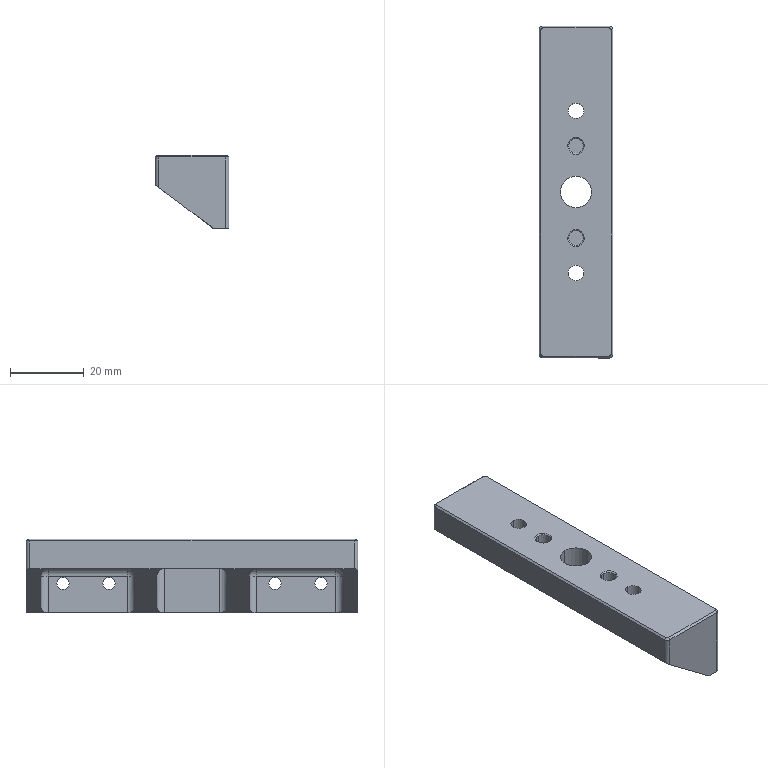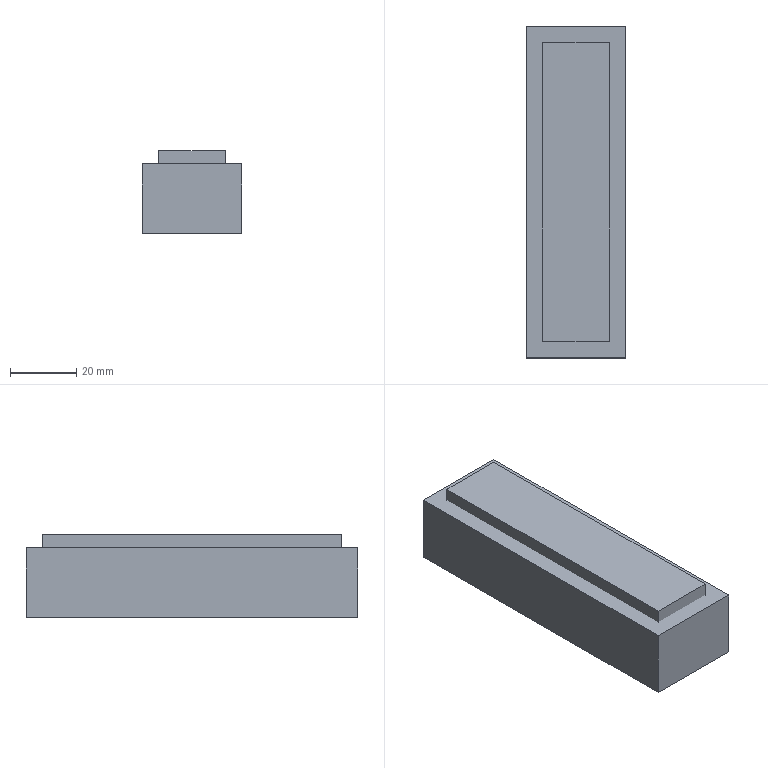CAM job | NX | 3+2 milling, drilling | part box 20 x 90 x 20 mm | stock box 30 x 100 x 25 mm
Tools:
number,name,description,diameter,corner_radius,flute_length,length,flutes
19,D80,Milling Tool-5 Parameters,80.0,0.0,50.0,75.0,2
1,D6A45,Milling Tool-5 Parameters,6.0,0.0,50.0,75.0,2
4,4.2ZT,Drilling Tool,4.2,0.0,35.0,50.0,2
15,D10,Milling Tool-5 Parameters,10.0,0.0,50.0,75.0,2
14,D10JING,Milling Tool-5 Parameters,10.0,0.0,50.0,75.0,2
12,D6,Milling Tool-5 Parameters,6.0,0.0,50.0,75.0,2
17,D3,Milling Tool-5 Parameters,3.0,0.0,50.0,75.0,2
18,D4R0.5,Milling Tool-5 Parameters,4.0,0.5,50.0,75.0,2
3,3.3ZT,Drilling Tool,3.3,0.0,35.0,50.0,2
Operations:
program,operation,operation_type,tool,method,geometry_group,spindle_rpm,surface_speed,feed_per_tooth,feed_cut,feed_plunge,cut_length_mm,path_length_mm,cut_time_min,machine_time_min
1,FLOOR_WALL,VolumeBased25DMillingOperation,D80,METHOD,A,6500.0,1633.0,0.1154,1500.0,100.0,192.0,246.0,0.128,0.1334
1,DRILLING_COPY_1,Operation,D6A45,METHOD,A,5000.0,94.0,0.035,350.0,0.0,26.5,170.635,0.0757,0.0901
1,DRILLING_COPY_COPY,Operation,4.2ZT,METHOD,A,2000.0,20.0,0.045,180.0,0.0,30.524,168.149,0.1696,0.1833
1,ADAPTIVE_MILLING,CavityMilling,D10,METHOD,A,9500.0,298.0,0.1579,3000.0,1000.0,1321.539,1415.539,0.4425,0.4519
1,ZLEVEL_PROFILE_COPY_1_COPY_COPY_1,ZLevelMilling,D10JING,METHOD,A,9500.0,298.0,0.0632,1200.0,1000.0,257.063,355.063,0.2148,0.2246
1,HOLE_MILLING,CylinderMilling,D6,METHOD,A,9500.0,179.0,0.0789,1500.0,100.0,145.569,213.069,0.097,0.1038
1,HOLE_MILLING_COPY,CylinderMilling,D3,METHOD,A,9500.0,89.0,0.0632,1200.0,100.0,138.875,294.875,0.1157,0.1313
1,PLANAR_MILL_COPY_COPY_COPY_COPY_COPY_COPY_1,PlanarMilling,D6A45,METHOD,A,9500.0,179.0,0.0658,1250.0,100.0,225.891,284.891,0.1807,0.1866
1,HOLE_MILLING_COPY_COPY,CylinderMilling,D3,METHOD,A,9500.0,89.0,0.0632,1200.0,100.0,26.316,182.316,0.0219,0.0375
2,FLOOR_WALL_COPY,VolumeBased25DMillingOperation,D80,METHOD,B,6500.0,1633.0,0.1154,1500.0,100.0,930.0,1900.001,0.62,0.717
2,CAVITY_MILL,CavityMilling,D10,METHOD,B,9500.0,298.0,0.1579,3000.0,1000.0,3951.136,4253.801,1.448,1.479
2,FIXED_CONTOUR,SurfaceContour,D4R0.5,METHOD,B,9500.0,119.0,0.1316,2500.0,1000.0,17954.208,18167.669,7.199,7.221
2,ZLEVEL_PROFILE,ZLevelMilling,D4R0.5,METHOD,B,9500.0,119.0,0.1842,3500.0,1000.0,5372.242,5780.51,1.552,1.593
3,DRILLING_COPY_1_COPY,Operation,D6A45,METHOD,C,5000.0,94.0,0.035,350.0,0.0,19.0,177.81,0.0543,0.0702
3,DRILLING_COPY_1_COPY_COPY,Operation,D6A45,METHOD,C,5000.0,94.0,0.035,350.0,0.0,10.6,109.379,0.0303,0.0402
3,DRILLING_COPY_COPY_COPY,Operation,3.3ZT,METHOD,C,2000.0,20.0,0.03,120.0,0.0,37.966,215.741,0.3164,0.3342
3,HOLE_MILLING_COPY_COPY_1,CylinderMilling,D3,METHOD,C,9500.0,89.0,0.0632,1200.0,100.0,110.637,262.637,0.0922,0.1074